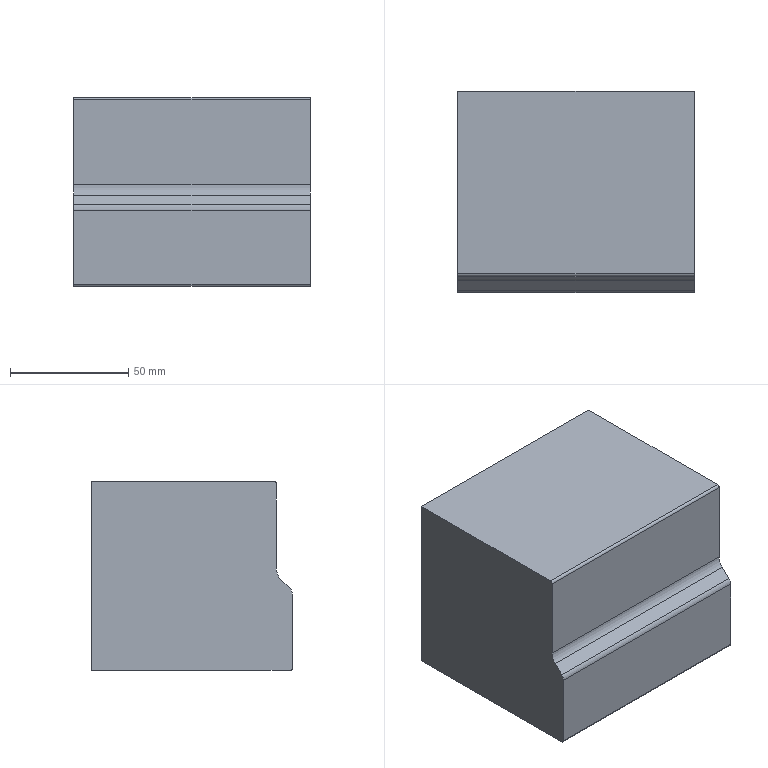Part | SolidWorks | features FlatPattern 1, ICE 1, SMBaseFlange 1, SheetMetal 1 | 1 solid | 15 faces | box 100 x 85 x 80 mm | volume 649829 mm3 | plane 9 | cylinder 6 | commonest cylinder face diameters 2 x2 16 x2 6.4 x1 12.8 x1
STEP:
#1=CARTESIAN_POINT('',(-50.,-5.,-48.));
#2=VERTEX_POINT('',#1);
#3=CARTESIAN_POINT('',(-50.,-5.,-32.));
#4=VERTEX_POINT('',#3);
#5=CARTESIAN_POINT('',(-50.,-5.,-40.));
#6=DIRECTION('',(0.,1.,0.));
#7=DIRECTION('',(0.,0.,1.));
#8=AXIS2_PLACEMENT_3D('',#5,#6,#7);
#9=CIRCLE('',#8,8.);
#10=EDGE_CURVE('',#2,#4,#9,.T.);
#11=ORIENTED_EDGE('',*,*,#10,.F.);
#12=CARTESIAN_POINT('',(-50.,0.,-48.));
#13=VERTEX_POINT('',#12);
#14=CARTESIAN_POINT('',(-50.,-5.,-48.));
#15=DIRECTION('',(0.,1.,0.));
#16=VECTOR('',#15,1000.);
#17=LINE('',#14,#16);
#18=EDGE_CURVE('',#2,#13,#17,.T.);
#19=ORIENTED_EDGE('',*,*,#18,.T.);
#20=CARTESIAN_POINT('',(-50.,0.,-32.));
#21=VERTEX_POINT('',#20);
#22=CARTESIAN_POINT('',(-50.,0.,-40.));
#23=DIRECTION('',(0.,1.,0.));
#24=DIRECTION('',(0.,0.,1.));
#25=AXIS2_PLACEMENT_3D('',#22,#23,#24);
#26=CIRCLE('',#25,8.);
#27=EDGE_CURVE('',#13,#21,#26,.T.);
#28=ORIENTED_EDGE('',*,*,#27,.T.);
#29=CARTESIAN_POINT('',(-50.,-5.,-32.));
#30=DIRECTION('',(0.,1.,0.));
#31=VECTOR('',#30,1000.);
#32=LINE('',#29,#31);
#33=EDGE_CURVE('',#4,#21,#32,.T.);
#34=ORIENTED_EDGE('',*,*,#33,.F.);
#35=EDGE_LOOP('',(#11,#19,#28,#34));
#36=FACE_OUTER_BOUND('',#35,.T.);
#37=CARTESIAN_POINT('',(-50.,-5.,-40.));
#38=DIRECTION('',(0.,1.,0.));
#39=DIRECTION('',(0.,0.,1.));
#40=AXIS2_PLACEMENT_3D('',#37,#38,#39);
#41=CYLINDRICAL_SURFACE('',#40,8.);
#42=ADVANCED_FACE('',(#36),#41,.F.);
#43=CARTESIAN_POINT('',(0.,0.,0.));
#44=VERTEX_POINT('',#43);
#45=CARTESIAN_POINT('',(0.,-77.2,0.));
#46=VERTEX_POINT('',#45);
#47=CARTESIAN_POINT('',(0.,-77.2,0.));
#48=DIRECTION('',(0.,-1.,0.));
#49=VECTOR('',#48,1000.);
#50=LINE('',#47,#49);
#51=EDGE_CURVE('',#44,#46,#50,.T.);
#52=ORIENTED_EDGE('',*,*,#51,.F.);
#53=CARTESIAN_POINT('',(-100.,0.,0.));
#54=VERTEX_POINT('',#53);
#55=CARTESIAN_POINT('',(-100.,0.,0.));
#56=DIRECTION('',(1.,0.,0.));
#57=VECTOR('',#56,1000.);
#58=LINE('',#55,#57);
#59=EDGE_CURVE('',#54,#44,#58,.T.);
#60=ORIENTED_EDGE('',*,*,#59,.F.);
#61=CARTESIAN_POINT('',(-100.,-77.2,0.));
#62=VERTEX_POINT('',#61);
#63=CARTESIAN_POINT('',(-100.,-77.2,0.));
#64=DIRECTION('',(0.,-1.,0.));
#65=VECTOR('',#64,1000.);
#66=LINE('',#63,#65);
#67=EDGE_CURVE('',#54,#62,#66,.T.);
#68=ORIENTED_EDGE('',*,*,#67,.T.);
#69=CARTESIAN_POINT('',(-100.,-77.2,0.));
#70=DIRECTION('',(1.,0.,0.));
#71=VECTOR('',#70,1000.);
#72=LINE('',#69,#71);
#73=EDGE_CURVE('',#62,#46,#72,.T.);
#74=ORIENTED_EDGE('',*,*,#73,.T.);
#75=EDGE_LOOP('',(#52,#60,#68,#74));
#76=FACE_OUTER_BOUND('',#75,.T.);
#77=CARTESIAN_POINT('',(-100.,-77.2,0.));
#78=DIRECTION('',(0.,0.,1.));
#79=DIRECTION('',(1.,0.,0.));
#80=AXIS2_PLACEMENT_3D('',#77,#78,#79);
#81=PLANE('',#80);
#82=ADVANCED_FACE('',(#76),#81,.T.);
#83=CARTESIAN_POINT('',(-50.,0.,-40.));
#84=DIRECTION('',(0.,1.,0.));
#85=DIRECTION('',(0.,0.,1.));
#86=AXIS2_PLACEMENT_3D('',#83,#84,#85);
#87=CIRCLE('',#86,8.);
#88=EDGE_CURVE('',#21,#13,#87,.T.);
#89=ORIENTED_EDGE('',*,*,#88,.F.);
#90=ORIENTED_EDGE('',*,*,#27,.F.);
#91=EDGE_LOOP('',(#89,#90));
#92=FACE_BOUND('',#91,.T.);
#93=CARTESIAN_POINT('',(0.,0.,-80.));
#94=VERTEX_POINT('',#93);
#95=CARTESIAN_POINT('',(0.,0.,0.));
#96=DIRECTION('',(0.,0.,1.));
#97=VECTOR('',#96,1000.);
#98=LINE('',#95,#97);
#99=EDGE_CURVE('',#94,#44,#98,.T.);
#100=ORIENTED_EDGE('',*,*,#99,.F.);
#101=CARTESIAN_POINT('',(-100.,0.,-80.));
#102=VERTEX_POINT('',#101);
#103=CARTESIAN_POINT('',(-100.,0.,-80.));
#104=DIRECTION('',(1.,0.,0.));
#105=VECTOR('',#104,1000.);
#106=LINE('',#103,#105);
#107=EDGE_CURVE('',#102,#94,#106,.T.);
#108=ORIENTED_EDGE('',*,*,#107,.F.);
#109=CARTESIAN_POINT('',(-100.,0.,0.));
#110=DIRECTION('',(0.,0.,1.));
#111=VECTOR('',#110,1000.);
#112=LINE('',#109,#111);
#113=EDGE_CURVE('',#102,#54,#112,.T.);
#114=ORIENTED_EDGE('',*,*,#113,.T.);
#115=ORIENTED_EDGE('',*,*,#59,.T.);
#116=EDGE_LOOP('',(#100,#108,#114,#115));
#117=FACE_OUTER_BOUND('',#116,.T.);
#118=CARTESIAN_POINT('',(-100.,0.,0.));
#119=DIRECTION('',(0.,1.,0.));
#120=DIRECTION('',(0.,0.,1.));
#121=AXIS2_PLACEMENT_3D('',#118,#119,#120);
#122=PLANE('',#121);
#123=ADVANCED_FACE('',(#92,#117),#122,.T.);
#124=CARTESIAN_POINT('',(0.,-84.,-80.));
#125=VERTEX_POINT('',#124);
#126=CARTESIAN_POINT('',(0.,0.,-80.));
#127=DIRECTION('',(0.,1.,0.));
#128=VECTOR('',#127,1000.);
#129=LINE('',#126,#128);
#130=EDGE_CURVE('',#125,#94,#129,.T.);
#131=ORIENTED_EDGE('',*,*,#130,.F.);
#132=CARTESIAN_POINT('',(-100.,-84.,-80.));
#133=VERTEX_POINT('',#132);
#134=CARTESIAN_POINT('',(-100.,-84.,-80.));
#135=DIRECTION('',(1.,0.,0.));
#136=VECTOR('',#135,1000.);
#137=LINE('',#134,#136);
#138=EDGE_CURVE('',#133,#125,#137,.T.);
#139=ORIENTED_EDGE('',*,*,#138,.F.);
#140=CARTESIAN_POINT('',(-100.,0.,-80.));
#141=DIRECTION('',(0.,1.,0.));
#142=VECTOR('',#141,1000.);
#143=LINE('',#140,#142);
#144=EDGE_CURVE('',#133,#102,#143,.T.);
#145=ORIENTED_EDGE('',*,*,#144,.T.);
#146=ORIENTED_EDGE('',*,*,#107,.T.);
#147=EDGE_LOOP('',(#131,#139,#145,#146));
#148=FACE_OUTER_BOUND('',#147,.T.);
#149=CARTESIAN_POINT('',(-100.,0.,-80.));
#150=DIRECTION('',(0.,0.,-1.));
#151=DIRECTION('',(0.,1.,0.));
#152=AXIS2_PLACEMENT_3D('',#149,#150,#151);
#153=PLANE('',#152);
#154=ADVANCED_FACE('',(#148),#153,.T.);
#155=CARTESIAN_POINT('',(0.,-85.,-79.));
#156=VERTEX_POINT('',#155);
#157=CARTESIAN_POINT('',(0.,-84.,-79.));
#158=DIRECTION('',(1.,0.,0.));
#159=DIRECTION('',(0.,0.,1.));
#160=AXIS2_PLACEMENT_3D('',#157,#158,#159);
#161=CIRCLE('',#160,1.);
#162=EDGE_CURVE('',#156,#125,#161,.T.);
#163=ORIENTED_EDGE('',*,*,#162,.F.);
#164=CARTESIAN_POINT('',(-100.,-85.,-79.));
#165=VERTEX_POINT('',#164);
#166=CARTESIAN_POINT('',(-100.,-85.,-79.));
#167=DIRECTION('',(1.,0.,0.));
#168=VECTOR('',#167,1000.);
#169=LINE('',#166,#168);
#170=EDGE_CURVE('',#165,#156,#169,.T.);
#171=ORIENTED_EDGE('',*,*,#170,.F.);
#172=CARTESIAN_POINT('',(-100.,-84.,-79.));
#173=DIRECTION('',(1.,0.,0.));
#174=DIRECTION('',(0.,0.,1.));
#175=AXIS2_PLACEMENT_3D('',#172,#173,#174);
#176=CIRCLE('',#175,1.);
#177=EDGE_CURVE('',#165,#133,#176,.T.);
#178=ORIENTED_EDGE('',*,*,#177,.T.);
#179=ORIENTED_EDGE('',*,*,#138,.T.);
#180=EDGE_LOOP('',(#163,#171,#178,#179));
#181=FACE_OUTER_BOUND('',#180,.T.);
#182=CARTESIAN_POINT('',(-100.,-84.,-79.));
#183=DIRECTION('',(1.,0.,0.));
#184=DIRECTION('',(0.,0.,-1.));
#185=AXIS2_PLACEMENT_3D('',#182,#183,#184);
#186=CYLINDRICAL_SURFACE('',#185,1.);
#187=ADVANCED_FACE('',(#181),#186,.T.);
#188=CARTESIAN_POINT('',(0.,-85.,-47.651));
#189=VERTEX_POINT('',#188);
#190=CARTESIAN_POINT('',(0.,-85.,-79.));
#191=DIRECTION('',(0.,0.,-1.));
#192=VECTOR('',#191,1000.);
#193=LINE('',#190,#192);
#194=EDGE_CURVE('',#189,#156,#193,.T.);
#195=ORIENTED_EDGE('',*,*,#194,.F.);
#196=CARTESIAN_POINT('',(-100.,-85.,-47.651));
#197=VERTEX_POINT('',#196);
#198=CARTESIAN_POINT('',(-100.,-85.,-47.651));
#199=DIRECTION('',(1.,0.,0.));
#200=VECTOR('',#199,1000.);
#201=LINE('',#198,#200);
#202=EDGE_CURVE('',#197,#189,#201,.T.);
#203=ORIENTED_EDGE('',*,*,#202,.F.);
#204=CARTESIAN_POINT('',(-100.,-85.,-79.));
#205=DIRECTION('',(0.,0.,-1.));
#206=VECTOR('',#205,1000.);
#207=LINE('',#204,#206);
#208=EDGE_CURVE('',#197,#165,#207,.T.);
#209=ORIENTED_EDGE('',*,*,#208,.T.);
#210=ORIENTED_EDGE('',*,*,#170,.T.);
#211=EDGE_LOOP('',(#195,#203,#209,#210));
#212=FACE_OUTER_BOUND('',#211,.T.);
#213=CARTESIAN_POINT('',(-100.,-85.,-79.));
#214=DIRECTION('',(0.,-1.,0.));
#215=DIRECTION('',(0.,0.,-1.));
#216=AXIS2_PLACEMENT_3D('',#213,#214,#215);
#217=PLANE('',#216);
#218=ADVANCED_FACE('',(#212),#217,.T.);
#219=CARTESIAN_POINT('',(0.,-84.063,-45.388));
#220=VERTEX_POINT('',#219);
#221=CARTESIAN_POINT('',(0.,-81.8,-47.651));
#222=DIRECTION('',(1.,0.,0.));
#223=DIRECTION('',(0.,0.,1.));
#224=AXIS2_PLACEMENT_3D('',#221,#222,#223);
#225=CIRCLE('',#224,3.2);
#226=EDGE_CURVE('',#220,#189,#225,.T.);
#227=ORIENTED_EDGE('',*,*,#226,.F.);
#228=CARTESIAN_POINT('',(-100.,-84.063,-45.388));
#229=VERTEX_POINT('',#228);
#230=CARTESIAN_POINT('',(-100.,-84.063,-45.388));
#231=DIRECTION('',(1.,0.,0.));
#232=VECTOR('',#231,1000.);
#233=LINE('',#230,#232);
#234=EDGE_CURVE('',#229,#220,#233,.T.);
#235=ORIENTED_EDGE('',*,*,#234,.F.);
#236=CARTESIAN_POINT('',(-100.,-81.8,-47.651));
#237=DIRECTION('',(1.,0.,0.));
#238=DIRECTION('',(0.,0.,1.));
#239=AXIS2_PLACEMENT_3D('',#236,#237,#238);
#240=CIRCLE('',#239,3.2);
#241=EDGE_CURVE('',#229,#197,#240,.T.);
#242=ORIENTED_EDGE('',*,*,#241,.T.);
#243=ORIENTED_EDGE('',*,*,#202,.T.);
#244=EDGE_LOOP('',(#227,#235,#242,#243));
#245=FACE_OUTER_BOUND('',#244,.T.);
#246=CARTESIAN_POINT('',(-100.,-81.8,-47.651));
#247=DIRECTION('',(1.,0.,0.));
#248=DIRECTION('',(0.,0.,-1.));
#249=AXIS2_PLACEMENT_3D('',#246,#247,#248);
#250=CYLINDRICAL_SURFACE('',#249,3.2);
#251=ADVANCED_FACE('',(#245),#250,.T.);
#252=CARTESIAN_POINT('',(0.,-80.075,-41.4));
#253=VERTEX_POINT('',#252);
#254=CARTESIAN_POINT('',(0.,-84.063,-45.388));
#255=DIRECTION('',(0.,-0.7071,-0.7071));
#256=VECTOR('',#255,1000.);
#257=LINE('',#254,#256);
#258=EDGE_CURVE('',#253,#220,#257,.T.);
#259=ORIENTED_EDGE('',*,*,#258,.F.);
#260=CARTESIAN_POINT('',(-100.,-80.075,-41.4));
#261=VERTEX_POINT('',#260);
#262=CARTESIAN_POINT('',(-100.,-80.075,-41.4));
#263=DIRECTION('',(1.,0.,0.));
#264=VECTOR('',#263,1000.);
#265=LINE('',#262,#264);
#266=EDGE_CURVE('',#261,#253,#265,.T.);
#267=ORIENTED_EDGE('',*,*,#266,.F.);
#268=CARTESIAN_POINT('',(-100.,-84.063,-45.388));
#269=DIRECTION('',(0.,-0.7071,-0.7071));
#270=VECTOR('',#269,1000.);
#271=LINE('',#268,#270);
#272=EDGE_CURVE('',#261,#229,#271,.T.);
#273=ORIENTED_EDGE('',*,*,#272,.T.);
#274=ORIENTED_EDGE('',*,*,#234,.T.);
#275=EDGE_LOOP('',(#259,#267,#273,#274));
#276=FACE_OUTER_BOUND('',#275,.T.);
#277=CARTESIAN_POINT('',(-100.,-84.063,-45.388));
#278=DIRECTION('',(0.,-0.7071,0.7071));
#279=DIRECTION('',(0.,-0.7071,-0.7071));
#280=AXIS2_PLACEMENT_3D('',#277,#278,#279);
#281=PLANE('',#280);
#282=ADVANCED_FACE('',(#276),#281,.T.);
#283=CARTESIAN_POINT('',(0.,-78.2,-36.875));
#284=VERTEX_POINT('',#283);
#285=CARTESIAN_POINT('',(0.,-84.6,-36.875));
#286=DIRECTION('',(-1.,0.,0.));
#287=DIRECTION('',(0.,0.,-1.));
#288=AXIS2_PLACEMENT_3D('',#285,#286,#287);
#289=CIRCLE('',#288,6.4);
#290=EDGE_CURVE('',#284,#253,#289,.T.);
#291=ORIENTED_EDGE('',*,*,#290,.F.);
#292=CARTESIAN_POINT('',(-100.,-78.2,-36.875));
#293=VERTEX_POINT('',#292);
#294=CARTESIAN_POINT('',(-100.,-78.2,-36.875));
#295=DIRECTION('',(1.,0.,0.));
#296=VECTOR('',#295,1000.);
#297=LINE('',#294,#296);
#298=EDGE_CURVE('',#293,#284,#297,.T.);
#299=ORIENTED_EDGE('',*,*,#298,.F.);
#300=CARTESIAN_POINT('',(-100.,-84.6,-36.875));
#301=DIRECTION('',(-1.,0.,0.));
#302=DIRECTION('',(0.,0.,-1.));
#303=AXIS2_PLACEMENT_3D('',#300,#301,#302);
#304=CIRCLE('',#303,6.4);
#305=EDGE_CURVE('',#293,#261,#304,.T.);
#306=ORIENTED_EDGE('',*,*,#305,.T.);
#307=ORIENTED_EDGE('',*,*,#266,.T.);
#308=EDGE_LOOP('',(#291,#299,#306,#307));
#309=FACE_OUTER_BOUND('',#308,.T.);
#310=CARTESIAN_POINT('',(-100.,-84.6,-36.875));
#311=DIRECTION('',(1.,0.,0.));
#312=DIRECTION('',(0.,0.,-1.));
#313=AXIS2_PLACEMENT_3D('',#310,#311,#312);
#314=CYLINDRICAL_SURFACE('',#313,6.4);
#315=ADVANCED_FACE('',(#309),#314,.F.);
#316=CARTESIAN_POINT('',(0.,-78.2,-1.));
#317=VERTEX_POINT('',#316);
#318=CARTESIAN_POINT('',(0.,-78.2,-36.875));
#319=DIRECTION('',(0.,0.,-1.));
#320=VECTOR('',#319,1000.);
#321=LINE('',#318,#320);
#322=EDGE_CURVE('',#317,#284,#321,.T.);
#323=ORIENTED_EDGE('',*,*,#322,.F.);
#324=CARTESIAN_POINT('',(-100.,-78.2,-1.));
#325=VERTEX_POINT('',#324);
#326=CARTESIAN_POINT('',(-100.,-78.2,-1.));
#327=DIRECTION('',(1.,0.,0.));
#328=VECTOR('',#327,1000.);
#329=LINE('',#326,#328);
#330=EDGE_CURVE('',#325,#317,#329,.T.);
#331=ORIENTED_EDGE('',*,*,#330,.F.);
#332=CARTESIAN_POINT('',(-100.,-78.2,-36.875));
#333=DIRECTION('',(0.,0.,-1.));
#334=VECTOR('',#333,1000.);
#335=LINE('',#332,#334);
#336=EDGE_CURVE('',#325,#293,#335,.T.);
#337=ORIENTED_EDGE('',*,*,#336,.T.);
#338=ORIENTED_EDGE('',*,*,#298,.T.);
#339=EDGE_LOOP('',(#323,#331,#337,#338));
#340=FACE_OUTER_BOUND('',#339,.T.);
#341=CARTESIAN_POINT('',(-100.,-78.2,-36.875));
#342=DIRECTION('',(0.,-1.,0.));
#343=DIRECTION('',(0.,0.,-1.));
#344=AXIS2_PLACEMENT_3D('',#341,#342,#343);
#345=PLANE('',#344);
#346=ADVANCED_FACE('',(#340),#345,.T.);
#347=CARTESIAN_POINT('',(0.,-77.2,-1.));
#348=DIRECTION('',(1.,0.,0.));
#349=DIRECTION('',(0.,0.,-1.));
#350=AXIS2_PLACEMENT_3D('',#347,#348,#349);
#351=CIRCLE('',#350,1.);
#352=EDGE_CURVE('',#46,#317,#351,.T.);
#353=ORIENTED_EDGE('',*,*,#352,.F.);
#354=ORIENTED_EDGE('',*,*,#73,.F.);
#355=CARTESIAN_POINT('',(-100.,-77.2,-1.));
#356=DIRECTION('',(1.,0.,0.));
#357=DIRECTION('',(0.,0.,-1.));
#358=AXIS2_PLACEMENT_3D('',#355,#356,#357);
#359=CIRCLE('',#358,1.);
#360=EDGE_CURVE('',#62,#325,#359,.T.);
#361=ORIENTED_EDGE('',*,*,#360,.T.);
#362=ORIENTED_EDGE('',*,*,#330,.T.);
#363=EDGE_LOOP('',(#353,#354,#361,#362));
#364=FACE_OUTER_BOUND('',#363,.T.);
#365=CARTESIAN_POINT('',(-100.,-77.2,-1.));
#366=DIRECTION('',(1.,0.,0.));
#367=DIRECTION('',(0.,0.,-1.));
#368=AXIS2_PLACEMENT_3D('',#365,#366,#367);
#369=CYLINDRICAL_SURFACE('',#368,1.);
#370=ADVANCED_FACE('',(#364),#369,.T.);
#371=ORIENTED_EDGE('',*,*,#67,.F.);
#372=ORIENTED_EDGE('',*,*,#113,.F.);
#373=ORIENTED_EDGE('',*,*,#144,.F.);
#374=ORIENTED_EDGE('',*,*,#177,.F.);
#375=ORIENTED_EDGE('',*,*,#208,.F.);
#376=ORIENTED_EDGE('',*,*,#241,.F.);
#377=ORIENTED_EDGE('',*,*,#272,.F.);
#378=ORIENTED_EDGE('',*,*,#305,.F.);
#379=ORIENTED_EDGE('',*,*,#336,.F.);
#380=ORIENTED_EDGE('',*,*,#360,.F.);
#381=EDGE_LOOP('',(#371,#372,#373,#374,#375,#376,#377,#378,#379,#380));
#382=FACE_OUTER_BOUND('',#381,.T.);
#383=CARTESIAN_POINT('',(-100.,-84.,-79.));
#384=DIRECTION('',(-1.,0.,0.));
#385=DIRECTION('',(0.,0.,1.));
#386=AXIS2_PLACEMENT_3D('',#383,#384,#385);
#387=PLANE('',#386);
#388=ADVANCED_FACE('',(#382),#387,.T.);
#389=ORIENTED_EDGE('',*,*,#51,.T.);
#390=ORIENTED_EDGE('',*,*,#352,.T.);
#391=ORIENTED_EDGE('',*,*,#322,.T.);
#392=ORIENTED_EDGE('',*,*,#290,.T.);
#393=ORIENTED_EDGE('',*,*,#258,.T.);
#394=ORIENTED_EDGE('',*,*,#226,.T.);
#395=ORIENTED_EDGE('',*,*,#194,.T.);
#396=ORIENTED_EDGE('',*,*,#162,.T.);
#397=ORIENTED_EDGE('',*,*,#130,.T.);
#398=ORIENTED_EDGE('',*,*,#99,.T.);
#399=EDGE_LOOP('',(#389,#390,#391,#392,#393,#394,#395,#396,#397,#398));
#400=FACE_OUTER_BOUND('',#399,.T.);
#401=CARTESIAN_POINT('',(0.,-84.,-79.));
#402=DIRECTION('',(-1.,0.,0.));
#403=DIRECTION('',(0.,0.,1.));
#404=AXIS2_PLACEMENT_3D('',#401,#402,#403);
#405=PLANE('',#404);
#406=ADVANCED_FACE('',(#400),#405,.F.);
#407=ORIENTED_EDGE('',*,*,#18,.F.);
#408=CARTESIAN_POINT('',(-50.,-5.,-40.));
#409=DIRECTION('',(0.,1.,0.));
#410=DIRECTION('',(0.,0.,1.));
#411=AXIS2_PLACEMENT_3D('',#408,#409,#410);
#412=CIRCLE('',#411,8.);
#413=EDGE_CURVE('',#4,#2,#412,.T.);
#414=ORIENTED_EDGE('',*,*,#413,.F.);
#415=ORIENTED_EDGE('',*,*,#33,.T.);
#416=ORIENTED_EDGE('',*,*,#88,.T.);
#417=EDGE_LOOP('',(#407,#414,#415,#416));
#418=FACE_OUTER_BOUND('',#417,.T.);
#419=CARTESIAN_POINT('',(-50.,-5.,-40.));
#420=DIRECTION('',(0.,1.,0.));
#421=DIRECTION('',(0.,0.,1.));
#422=AXIS2_PLACEMENT_3D('',#419,#420,#421);
#423=CYLINDRICAL_SURFACE('',#422,8.);
#424=ADVANCED_FACE('',(#418),#423,.F.);
#425=ORIENTED_EDGE('',*,*,#413,.T.);
#426=ORIENTED_EDGE('',*,*,#10,.T.);
#427=EDGE_LOOP('',(#425,#426));
#428=FACE_OUTER_BOUND('',#427,.T.);
#429=CARTESIAN_POINT('',(-50.,-5.,-40.));
#430=DIRECTION('',(0.,1.,0.));
#431=DIRECTION('',(0.,0.,1.));
#432=AXIS2_PLACEMENT_3D('',#429,#430,#431);
#433=PLANE('',#432);
#434=ADVANCED_FACE('',(#428),#433,.T.);
#435=CLOSED_SHELL('',(#42,#82,#123,#154,#187,#218,#251,#282,#315,#346,#370,#388,#406,#424,#434));
#436=MANIFOLD_SOLID_BREP('',#435);
#437=CARTESIAN_POINT('',(0.,0.,0.));
#438=DIRECTION('',(0.,0.,1.));
#439=DIRECTION('',(1.,0.,0.));
#440=AXIS2_PLACEMENT_3D('',#437,#438,#439);
#441=(LENGTH_UNIT()NAMED_UNIT(*)SI_UNIT(.MILLI.,.METRE.));
#442=UNCERTAINTY_MEASURE_WITH_UNIT(LENGTH_MEASURE(0.00001),#441,'','');
#443=(NAMED_UNIT(*)PLANE_ANGLE_UNIT()SI_UNIT($,.RADIAN.));
#444=(NAMED_UNIT(*)SI_UNIT($,.STERADIAN.)SOLID_ANGLE_UNIT());
#445=(GEOMETRIC_REPRESENTATION_CONTEXT(3)GLOBAL_UNCERTAINTY_ASSIGNED_CONTEXT((#442))GLOBAL_UNIT_ASSIGNED_CONTEXT((#441,#443,#444))REPRESENTATION_CONTEXT('',''));
#446=ADVANCED_BREP_SHAPE_REPRESENTATION('',(#436,#440),#445);